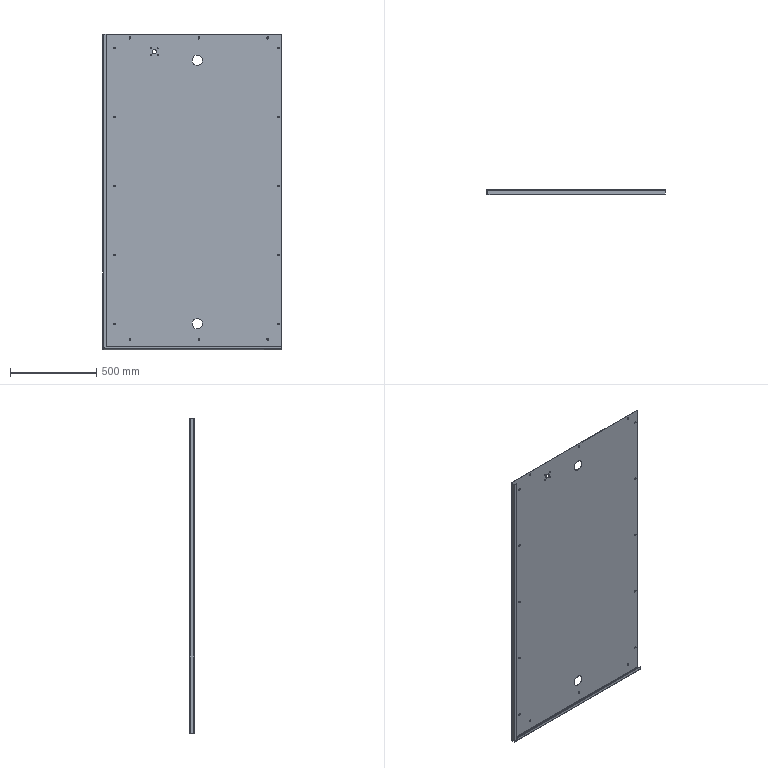Part | NX | features BREP 1 | 1 solid | 122 faces | box 1038 x 30 x 1830 mm | volume 3029199 mm3 | cylinder 60 | plane 58 | spline 4 | commonest cylinder face diameters 7 x42 6 x8 4 x4 60 x4 25 x2